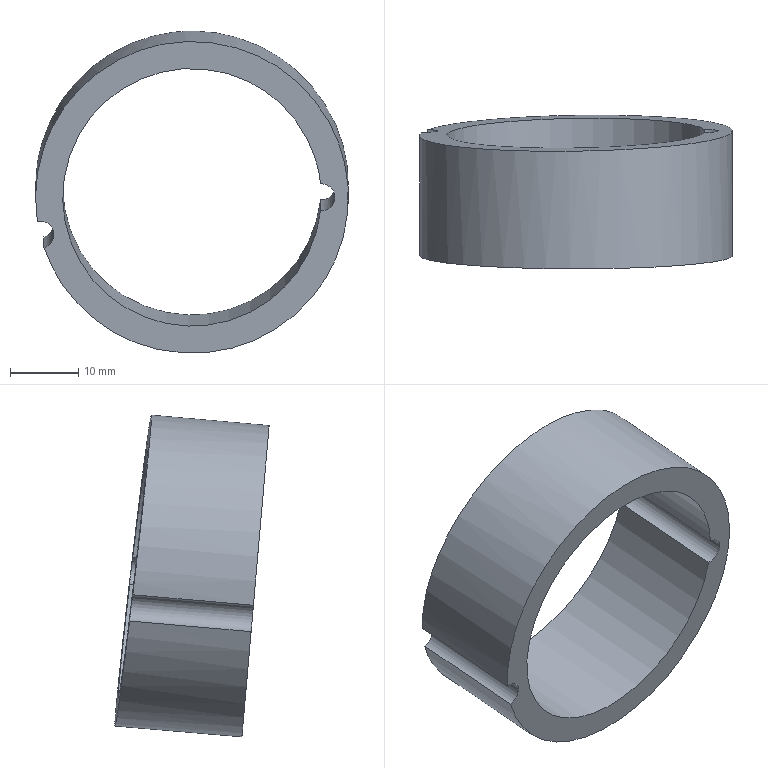Part | NX | features solid 2 | 1 solid | 6 faces | box 45.995 x 22.663 x 47.314 mm | volume 9277 mm3 | spline 2 | plane 2 | cylinder 2 | commonest cylinder face diameters 4 x2
STEP:
#1=CARTESIAN_POINT('',(-131.293,58.518,-39.778));
#2=VERTEX_POINT('',#1);
#3=CARTESIAN_POINT('',(-131.293,58.054,-35.809));
#4=VERTEX_POINT('',#3);
#5=CARTESIAN_POINT('',(-131.293,58.518,-39.778));
#6=CARTESIAN_POINT('',(-131.796,59.064,-44.514));
#7=CARTESIAN_POINT('',(-136.604,60.053,-53.6));
#8=CARTESIAN_POINT('',(-151.271,60.411,-58.575));
#9=CARTESIAN_POINT('',(-165.362,59.444,-52.144));
#10=CARTESIAN_POINT('',(-171.101,57.684,-37.845));
#11=CARTESIAN_POINT('',(-165.357,56.097,-23.527));
#12=CARTESIAN_POINT('',(-151.257,55.556,-17.065));
#13=CARTESIAN_POINT('',(-136.601,56.358,-22.008));
#14=CARTESIAN_POINT('',(-131.798,57.492,-31.074));
#15=CARTESIAN_POINT('',(-131.293,58.054,-35.809));
#16=B_SPLINE_CURVE_WITH_KNOTS('',3,(#5,#6,#7,#8,#9,#10,#11,#12,#13,#14,#15),.UNSPECIFIED.,.F.,.F.,(4,1,1,1,1,1,1,1,4),(0.05948,0.07384,0.08819,0.1025,0.1169,0.1313,0.1456,0.16,0.1743),.UNSPECIFIED.);
#17=EDGE_CURVE('',#2,#4,#16,.T.);
#18=ORIENTED_EDGE('',*,*,#17,.T.);
#19=CARTESIAN_POINT('',(-131.293,39.862,-37.401));
#20=VERTEX_POINT('',#19);
#21=CARTESIAN_POINT('',(-131.293,49.213,-36.583));
#22=DIRECTION('',(0.,0.9962,0.08716));
#23=VECTOR('',#22,1000.);
#24=LINE('',#21,#23);
#25=EDGE_CURVE('',#4,#20,#24,.F.);
#26=ORIENTED_EDGE('',*,*,#25,.T.);
#27=CARTESIAN_POINT('',(-131.293,40.21,-41.38));
#28=VERTEX_POINT('',#27);
#29=CARTESIAN_POINT('',(-131.293,40.21,-41.38));
#30=CARTESIAN_POINT('',(-131.797,40.626,-46.134));
#31=CARTESIAN_POINT('',(-136.612,41.423,-55.239));
#32=CARTESIAN_POINT('',(-151.288,41.857,-60.196));
#33=CARTESIAN_POINT('',(-165.36,41.291,-53.73));
#34=CARTESIAN_POINT('',(-171.101,40.036,-39.391));
#35=CARTESIAN_POINT('',(-165.36,38.782,-25.052));
#36=CARTESIAN_POINT('',(-151.289,38.216,-18.585));
#37=CARTESIAN_POINT('',(-136.612,38.65,-23.542));
#38=CARTESIAN_POINT('',(-131.799,39.446,-32.646));
#39=CARTESIAN_POINT('',(-131.293,39.862,-37.401));
#40=B_SPLINE_CURVE_WITH_KNOTS('',3,(#29,#30,#31,#32,#33,#34,#35,#36,#37,#38,#39),.UNSPECIFIED.,.F.,.F.,(4,1,1,1,1,1,1,1,4),(0.,0.1208,0.2416,0.3624,0.4832,0.604,0.7249,0.8457,0.9665),.UNSPECIFIED.);
#41=EDGE_CURVE('',#28,#20,#40,.T.);
#42=ORIENTED_EDGE('',*,*,#41,.F.);
#43=CARTESIAN_POINT('',(-131.293,49.561,-40.562));
#44=DIRECTION('',(0.,0.9962,0.08716));
#45=VECTOR('',#44,1000.);
#46=LINE('',#43,#45);
#47=EDGE_CURVE('',#28,#2,#46,.T.);
#48=ORIENTED_EDGE('',*,*,#47,.T.);
#49=EDGE_LOOP('',(#18,#26,#42,#48));
#50=FACE_BOUND('',#49,.T.);
#51=CARTESIAN_POINT('',(-131.293,40.21,-41.38));
#52=CARTESIAN_POINT('',(-131.293,58.912,-39.744));
#53=CARTESIAN_POINT('',(-131.797,40.626,-46.134));
#54=CARTESIAN_POINT('',(-131.797,59.328,-44.497));
#55=CARTESIAN_POINT('',(-136.612,41.423,-55.239));
#56=CARTESIAN_POINT('',(-136.612,60.124,-53.603));
#57=CARTESIAN_POINT('',(-151.288,41.857,-60.196));
#58=CARTESIAN_POINT('',(-151.288,60.558,-58.56));
#59=CARTESIAN_POINT('',(-165.36,41.291,-53.73));
#60=CARTESIAN_POINT('',(-165.36,59.992,-52.094));
#61=CARTESIAN_POINT('',(-171.101,40.036,-39.391));
#62=CARTESIAN_POINT('',(-171.101,58.738,-37.755));
#63=CARTESIAN_POINT('',(-165.36,38.782,-25.052));
#64=CARTESIAN_POINT('',(-165.36,57.483,-23.416));
#65=CARTESIAN_POINT('',(-151.289,38.216,-18.585));
#66=CARTESIAN_POINT('',(-151.289,56.917,-16.949));
#67=CARTESIAN_POINT('',(-136.612,38.65,-23.542));
#68=CARTESIAN_POINT('',(-136.612,57.351,-21.906));
#69=CARTESIAN_POINT('',(-131.799,39.446,-32.646));
#70=CARTESIAN_POINT('',(-131.799,58.148,-31.01));
#71=CARTESIAN_POINT('',(-131.293,39.862,-37.401));
#72=CARTESIAN_POINT('',(-131.293,58.564,-35.765));
#73=B_SPLINE_SURFACE_WITH_KNOTS('',3,1,((#51,#52),(#53,#54),(#55,#56),(#57,#58),(#59,#60),(#61,#62),(#63,#64),(#65,#66),(#67,#68),(#69,#70),(#71,#72)),.SURF_OF_LINEAR_EXTRUSION.,.F.,.F.,.F.,(4,1,1,1,1,1,1,1,4),(2,2),(0.,0.1208,0.2416,0.3624,0.4832,0.604,0.7249,0.8457,0.9665),(0.,1.),.UNSPECIFIED.);
#74=ADVANCED_FACE('',(#50),#73,.F.);
#75=CARTESIAN_POINT('',(-172.913,40.345,-42.914));
#76=VERTEX_POINT('',#75);
#77=CARTESIAN_POINT('',(-171.958,40.683,-46.782));
#78=VERTEX_POINT('',#77);
#79=CARTESIAN_POINT('',(-172.498,40.515,-44.863));
#80=DIRECTION('',(0.,0.9962,0.08716));
#81=DIRECTION('',(-1.,0.,0.));
#82=AXIS2_PLACEMENT_3D('',#79,#80,#81);
#83=CIRCLE('',#82,2.);
#84=EDGE_CURVE('',#76,#78,#83,.T.);
#85=ORIENTED_EDGE('',*,*,#84,.T.);
#86=CARTESIAN_POINT('',(-172.913,40.345,-42.914));
#87=CARTESIAN_POINT('',(-173.814,39.841,-37.153));
#88=CARTESIAN_POINT('',(-170.971,38.773,-24.947));
#89=CARTESIAN_POINT('',(-155.172,37.87,-14.634));
#90=CARTESIAN_POINT('',(-136.602,38.172,-18.076));
#91=CARTESIAN_POINT('',(-125.579,39.508,-33.353));
#92=CARTESIAN_POINT('',(-128.219,41.138,-51.985));
#93=CARTESIAN_POINT('',(-143.063,42.156,-63.623));
#94=CARTESIAN_POINT('',(-161.863,41.997,-61.796));
#95=CARTESIAN_POINT('',(-170.071,41.166,-52.303));
#96=CARTESIAN_POINT('',(-171.958,40.683,-46.782));
#97=B_SPLINE_CURVE_WITH_KNOTS('',3,(#86,#87,#88,#89,#90,#91,#92,#93,#94,#95,#96),.UNSPECIFIED.,.F.,.F.,(4,1,1,1,1,1,1,1,4),(0.4587,0.5802,0.7017,0.8233,0.9448,1.066,1.188,1.309,1.431),.UNSPECIFIED.);
#98=EDGE_CURVE('',#76,#78,#97,.T.);
#99=ORIENTED_EDGE('',*,*,#98,.F.);
#100=EDGE_LOOP('',(#85,#99));
#101=FACE_BOUND('',#100,.T.);
#102=CARTESIAN_POINT('',(-131.187,40.036,-39.391));
#103=DIRECTION('',(0.,0.9962,0.08716));
#104=DIRECTION('',(-1.,0.,0.));
#105=AXIS2_PLACEMENT_3D('',#102,#103,#104);
#106=CIRCLE('',#105,2.);
#107=EDGE_CURVE('',#20,#28,#106,.T.);
#108=ORIENTED_EDGE('',*,*,#107,.T.);
#109=ORIENTED_EDGE('',*,*,#41,.T.);
#110=EDGE_LOOP('',(#108,#109));
#111=FACE_BOUND('',#110,.T.);
#112=CARTESIAN_POINT('',(-128.309,40.238,-41.694));
#113=DIRECTION('',(0.,-0.9962,-0.08716));
#114=DIRECTION('',(0.,0.08716,-0.9962));
#115=AXIS2_PLACEMENT_3D('',#112,#113,#114);
#116=PLANE('',#115);
#117=ADVANCED_FACE('',(#101,#111),#116,.T.);
#118=CARTESIAN_POINT('',(-171.958,58.533,-45.22));
#119=VERTEX_POINT('',#118);
#120=CARTESIAN_POINT('',(-172.913,58.068,-41.364));
#121=VERTEX_POINT('',#120);
#122=CARTESIAN_POINT('',(-172.498,58.301,-43.307));
#123=DIRECTION('',(-0.01517,0.9931,0.1162));
#124=DIRECTION('',(-0.4611,-0.11,0.8805));
#125=AXIS2_PLACEMENT_3D('',#122,#123,#124);
#126=ELLIPSE('',#125,2.001,2.);
#127=EDGE_CURVE('',#119,#121,#126,.F.);
#128=ORIENTED_EDGE('',*,*,#127,.T.);
#129=CARTESIAN_POINT('',(-172.913,58.068,-41.364));
#130=CARTESIAN_POINT('',(-173.364,57.724,-38.484));
#131=CARTESIAN_POINT('',(-173.136,57.03,-32.52));
#132=CARTESIAN_POINT('',(-169.495,56.139,-24.426));
#133=CARTESIAN_POINT('',(-163.075,55.512,-18.232));
#134=CARTESIAN_POINT('',(-154.797,55.244,-14.863));
#135=CARTESIAN_POINT('',(-145.855,55.373,-14.797));
#136=CARTESIAN_POINT('',(-137.531,55.881,-18.051));
#137=CARTESIAN_POINT('',(-131.037,56.694,-24.15));
#138=CARTESIAN_POINT('',(-127.304,57.693,-32.21));
#139=CARTESIAN_POINT('',(-126.856,58.737,-41.075));
#140=CARTESIAN_POINT('',(-129.765,59.675,-49.473));
#141=CARTESIAN_POINT('',(-135.61,60.372,-56.197));
#142=CARTESIAN_POINT('',(-143.557,60.729,-60.28));
#143=CARTESIAN_POINT('',(-152.464,60.692,-61.13));
#144=CARTESIAN_POINT('',(-161.049,60.267,-58.613));
#145=CARTESIAN_POINT('',(-168.057,59.516,-53.109));
#146=CARTESIAN_POINT('',(-171.018,58.868,-47.961));
#147=CARTESIAN_POINT('',(-171.958,58.533,-45.22));
#148=B_SPLINE_CURVE_WITH_KNOTS('',3,(#129,#130,#131,#132,#133,#134,#135,#136,#137,#138,#139,#140,#141,#142,#143,#144,#145,#146,#147),.UNSPECIFIED.,.F.,.F.,(4,1,1,1,1,1,1,1,1,1,1,1,1,1,1,1,4),(0.138,0.1467,0.1555,0.1642,0.1729,0.1817,0.1904,0.1992,0.2079,0.2166,0.2254,0.2341,0.2429,0.2516,0.2603,0.2691,0.2778),.UNSPECIFIED.);
#149=EDGE_CURVE('',#121,#119,#148,.T.);
#150=ORIENTED_EDGE('',*,*,#149,.T.);
#151=EDGE_LOOP('',(#128,#150));
#152=FACE_BOUND('',#151,.T.);
#153=CARTESIAN_POINT('',(-131.187,58.287,-37.794));
#154=DIRECTION('',(-0.01517,0.9931,0.1162));
#155=DIRECTION('',(-0.4611,-0.11,0.8805));
#156=AXIS2_PLACEMENT_3D('',#153,#154,#155);
#157=ELLIPSE('',#156,2.001,2.);
#158=EDGE_CURVE('',#2,#4,#157,.F.);
#159=ORIENTED_EDGE('',*,*,#158,.T.);
#160=ORIENTED_EDGE('',*,*,#17,.F.);
#161=EDGE_LOOP('',(#159,#160));
#162=FACE_BOUND('',#161,.T.);
#163=CARTESIAN_POINT('',(-173.425,42.623,90.607));
#164=DIRECTION('',(-0.01517,0.9931,0.1162));
#165=DIRECTION('',(0.05188,0.1168,-0.9918));
#166=AXIS2_PLACEMENT_3D('',#163,#164,#165);
#167=PLANE('',#166);
#168=ADVANCED_FACE('',(#152,#162),#167,.T.);
#169=CARTESIAN_POINT('',(-171.958,50.1,-45.958));
#170=DIRECTION('',(0.,0.9962,0.08716));
#171=VECTOR('',#170,1000.);
#172=LINE('',#169,#171);
#173=EDGE_CURVE('',#119,#78,#172,.F.);
#174=ORIENTED_EDGE('',*,*,#173,.F.);
#175=ORIENTED_EDGE('',*,*,#149,.F.);
#176=CARTESIAN_POINT('',(-172.913,49.762,-42.09));
#177=DIRECTION('',(0.,0.9962,0.08716));
#178=VECTOR('',#177,1000.);
#179=LINE('',#176,#178);
#180=EDGE_CURVE('',#76,#121,#179,.T.);
#181=ORIENTED_EDGE('',*,*,#180,.F.);
#182=ORIENTED_EDGE('',*,*,#98,.T.);
#183=EDGE_LOOP('',(#174,#175,#181,#182));
#184=FACE_BOUND('',#183,.T.);
#185=CARTESIAN_POINT('',(-172.913,40.345,-42.914));
#186=CARTESIAN_POINT('',(-172.913,59.179,-41.266));
#187=CARTESIAN_POINT('',(-173.814,39.841,-37.153));
#188=CARTESIAN_POINT('',(-173.814,58.675,-35.505));
#189=CARTESIAN_POINT('',(-170.971,38.773,-24.947));
#190=CARTESIAN_POINT('',(-170.971,57.607,-23.3));
#191=CARTESIAN_POINT('',(-155.172,37.87,-14.634));
#192=CARTESIAN_POINT('',(-155.172,56.704,-12.986));
#193=CARTESIAN_POINT('',(-136.602,38.172,-18.076));
#194=CARTESIAN_POINT('',(-136.602,57.006,-16.428));
#195=CARTESIAN_POINT('',(-125.579,39.508,-33.353));
#196=CARTESIAN_POINT('',(-125.579,58.342,-31.705));
#197=CARTESIAN_POINT('',(-128.219,41.138,-51.985));
#198=CARTESIAN_POINT('',(-128.219,59.972,-50.337));
#199=CARTESIAN_POINT('',(-143.063,42.156,-63.623));
#200=CARTESIAN_POINT('',(-143.063,60.99,-61.975));
#201=CARTESIAN_POINT('',(-161.863,41.997,-61.796));
#202=CARTESIAN_POINT('',(-161.863,60.831,-60.148));
#203=CARTESIAN_POINT('',(-170.071,41.166,-52.303));
#204=CARTESIAN_POINT('',(-170.071,60.,-50.655));
#205=CARTESIAN_POINT('',(-171.958,40.683,-46.782));
#206=CARTESIAN_POINT('',(-171.958,59.517,-45.134));
#207=B_SPLINE_SURFACE_WITH_KNOTS('',3,1,((#185,#186),(#187,#188),(#189,#190),(#191,#192),(#193,#194),(#195,#196),(#197,#198),(#199,#200),(#201,#202),(#203,#204),(#205,#206)),.SURF_OF_LINEAR_EXTRUSION.,.F.,.F.,.F.,(4,1,1,1,1,1,1,1,4),(2,2),(0.4587,0.5802,0.7017,0.8233,0.9448,1.066,1.188,1.309,1.431),(0.,1.),.UNSPECIFIED.);
#208=ADVANCED_FACE('',(#184),#207,.T.);
#209=ORIENTED_EDGE('',*,*,#158,.F.);
#210=ORIENTED_EDGE('',*,*,#47,.F.);
#211=ORIENTED_EDGE('',*,*,#107,.F.);
#212=ORIENTED_EDGE('',*,*,#25,.F.);
#213=EDGE_LOOP('',(#209,#210,#211,#212));
#214=FACE_BOUND('',#213,.T.);
#215=CARTESIAN_POINT('',(-131.187,59.96,-37.647));
#216=DIRECTION('',(0.,-0.9962,-0.08716));
#217=DIRECTION('',(1.,0.,0.));
#218=AXIS2_PLACEMENT_3D('',#215,#216,#217);
#219=CYLINDRICAL_SURFACE('',#218,2.);
#220=ADVANCED_FACE('',(#214),#219,.F.);
#221=ORIENTED_EDGE('',*,*,#173,.T.);
#222=ORIENTED_EDGE('',*,*,#84,.F.);
#223=ORIENTED_EDGE('',*,*,#180,.T.);
#224=ORIENTED_EDGE('',*,*,#127,.F.);
#225=EDGE_LOOP('',(#221,#222,#223,#224));
#226=FACE_BOUND('',#225,.T.);
#227=CARTESIAN_POINT('',(-172.498,60.439,-43.12));
#228=DIRECTION('',(0.,-0.9962,-0.08716));
#229=DIRECTION('',(1.,0.,0.));
#230=AXIS2_PLACEMENT_3D('',#227,#228,#229);
#231=CYLINDRICAL_SURFACE('',#230,2.);
#232=ADVANCED_FACE('',(#226),#231,.F.);
#233=CLOSED_SHELL('',(#74,#117,#168,#208,#220,#232));
#234=MANIFOLD_SOLID_BREP('',#233);
#235=(LENGTH_UNIT()NAMED_UNIT(*)SI_UNIT(.MILLI.,.METRE.));
#236=UNCERTAINTY_MEASURE_WITH_UNIT(LENGTH_MEASURE(0.0508),#235,'','');
#237=(NAMED_UNIT(*)PLANE_ANGLE_UNIT()SI_UNIT($,.RADIAN.));
#238=(NAMED_UNIT(*)SI_UNIT($,.STERADIAN.)SOLID_ANGLE_UNIT());
#239=(GEOMETRIC_REPRESENTATION_CONTEXT(3)GLOBAL_UNCERTAINTY_ASSIGNED_CONTEXT((#236))GLOBAL_UNIT_ASSIGNED_CONTEXT((#235,#237,#238))REPRESENTATION_CONTEXT('',''));
#240=ADVANCED_BREP_SHAPE_REPRESENTATION('',(#234),#239);